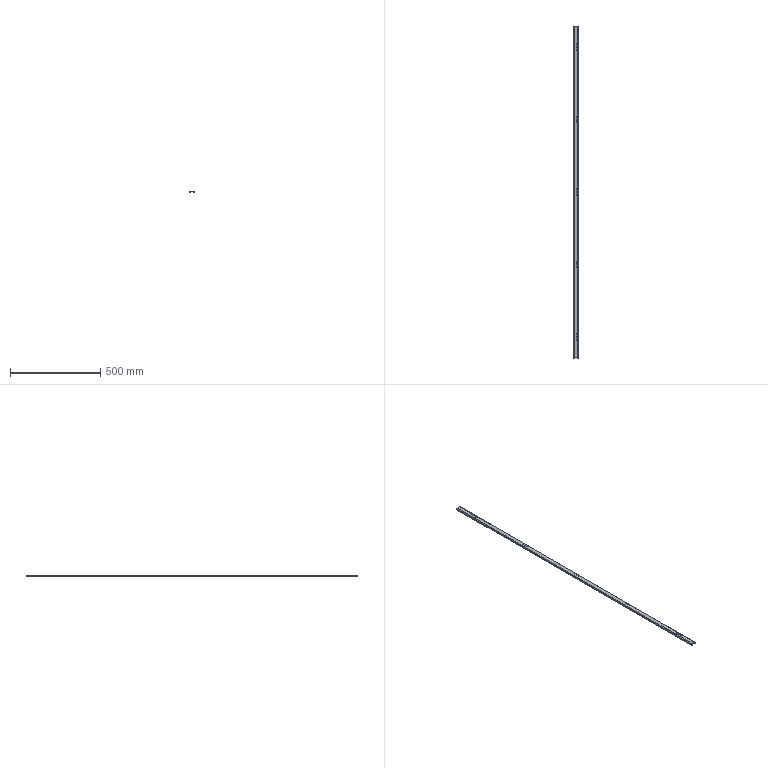Part | SolidWorks | features BaseBody 1 | 1 solid | 52 faces | box 27 x 1838 x 10 mm | volume 215628 mm3 | cylinder 34 | plane 18 | commonest cylinder face diameters 5.2 x30 1 x2 7 x2